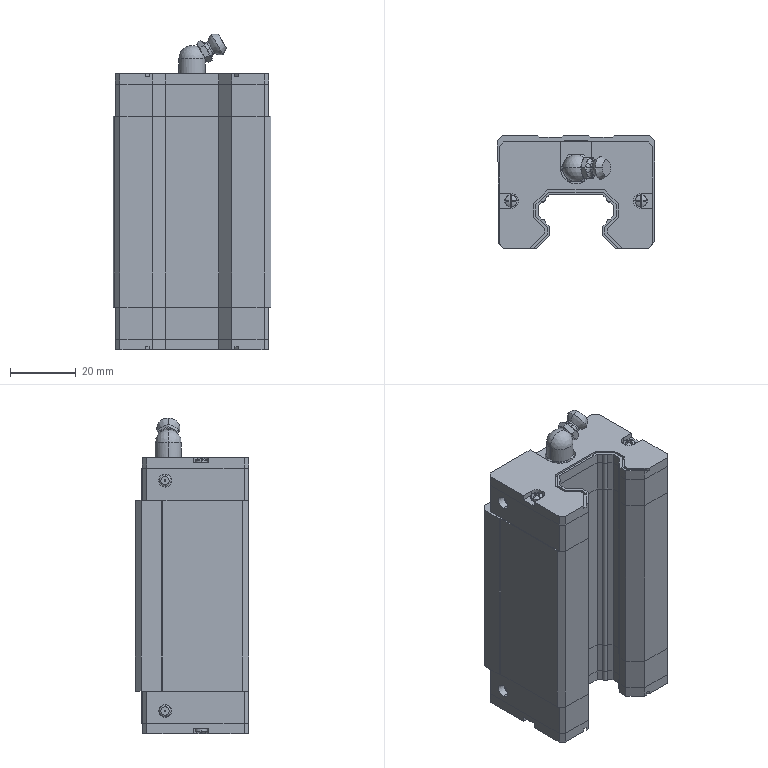Part | STEP file | 6 solids | 648 faces | box 48 x 34.4 x 96 mm | volume 105086 mm3 | plane 403 | spline 93 | cylinder 86 | cone 31 | torus 23 | sphere 10 | other 2 | commonest cylinder face diameters 2.258 x30 3.9 x12 0.526 x8 3.725 x8 4.8 x8 6 x8